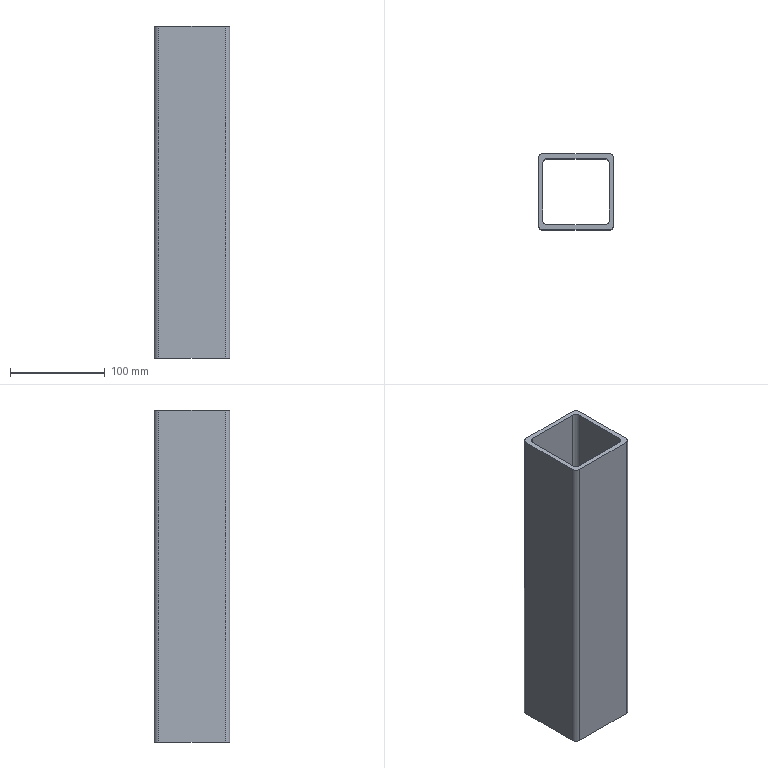Part | SolidWorks | features BaseBody 1 | 1 solid | 18 faces | box 80 x 80 x 350 mm | volume 525000 mm3 | plane 10 | cylinder 8 | commonest cylinder face diameters 10 x8
STEP:
#1=CARTESIAN_POINT('',(-40.,-35.,175.));
#2=VERTEX_POINT('',#1);
#3=CARTESIAN_POINT('',(-35.,-40.,175.));
#4=VERTEX_POINT('',#3);
#5=CARTESIAN_POINT('',(-35.,-35.,175.));
#6=DIRECTION('',(0.,0.,1.));
#7=DIRECTION('',(-1.,0.,0.));
#8=AXIS2_PLACEMENT_3D('',#5,#6,#7);
#9=CIRCLE('',#8,5.);
#10=EDGE_CURVE('',#2,#4,#9,.T.);
#11=ORIENTED_EDGE('',*,*,#10,.T.);
#12=CARTESIAN_POINT('',(35.,-40.,175.));
#13=VERTEX_POINT('',#12);
#14=CARTESIAN_POINT('',(35.,-40.,175.));
#15=DIRECTION('',(1.,0.,0.));
#16=VECTOR('',#15,1000.);
#17=LINE('',#14,#16);
#18=EDGE_CURVE('',#4,#13,#17,.T.);
#19=ORIENTED_EDGE('',*,*,#18,.T.);
#20=CARTESIAN_POINT('',(40.,-35.,175.));
#21=VERTEX_POINT('',#20);
#22=CARTESIAN_POINT('',(35.,-35.,175.));
#23=DIRECTION('',(0.,0.,1.));
#24=DIRECTION('',(1.,0.,0.));
#25=AXIS2_PLACEMENT_3D('',#22,#23,#24);
#26=CIRCLE('',#25,5.);
#27=EDGE_CURVE('',#13,#21,#26,.T.);
#28=ORIENTED_EDGE('',*,*,#27,.T.);
#29=CARTESIAN_POINT('',(40.,35.,175.));
#30=VERTEX_POINT('',#29);
#31=CARTESIAN_POINT('',(40.,-35.,175.));
#32=DIRECTION('',(0.,1.,0.));
#33=VECTOR('',#32,1000.);
#34=LINE('',#31,#33);
#35=EDGE_CURVE('',#21,#30,#34,.T.);
#36=ORIENTED_EDGE('',*,*,#35,.T.);
#37=CARTESIAN_POINT('',(35.,40.,175.));
#38=VERTEX_POINT('',#37);
#39=CARTESIAN_POINT('',(35.,35.,175.));
#40=DIRECTION('',(0.,0.,1.));
#41=DIRECTION('',(1.,0.,0.));
#42=AXIS2_PLACEMENT_3D('',#39,#40,#41);
#43=CIRCLE('',#42,5.);
#44=EDGE_CURVE('',#30,#38,#43,.T.);
#45=ORIENTED_EDGE('',*,*,#44,.T.);
#46=CARTESIAN_POINT('',(-35.,40.,175.));
#47=VERTEX_POINT('',#46);
#48=CARTESIAN_POINT('',(35.,40.,175.));
#49=DIRECTION('',(-1.,0.,0.));
#50=VECTOR('',#49,1000.);
#51=LINE('',#48,#50);
#52=EDGE_CURVE('',#38,#47,#51,.T.);
#53=ORIENTED_EDGE('',*,*,#52,.T.);
#54=CARTESIAN_POINT('',(-40.,35.,175.));
#55=VERTEX_POINT('',#54);
#56=CARTESIAN_POINT('',(-35.,35.,175.));
#57=DIRECTION('',(0.,0.,1.));
#58=DIRECTION('',(1.,0.,0.));
#59=AXIS2_PLACEMENT_3D('',#56,#57,#58);
#60=CIRCLE('',#59,5.);
#61=EDGE_CURVE('',#47,#55,#60,.T.);
#62=ORIENTED_EDGE('',*,*,#61,.T.);
#63=CARTESIAN_POINT('',(-40.,-35.,175.));
#64=DIRECTION('',(0.,-1.,0.));
#65=VECTOR('',#64,1000.);
#66=LINE('',#63,#65);
#67=EDGE_CURVE('',#55,#2,#66,.T.);
#68=ORIENTED_EDGE('',*,*,#67,.T.);
#69=EDGE_LOOP('',(#11,#19,#28,#36,#45,#53,#62,#68));
#70=FACE_OUTER_BOUND('',#69,.T.);
#71=CARTESIAN_POINT('',(-35.,-30.,175.));
#72=VERTEX_POINT('',#71);
#73=CARTESIAN_POINT('',(-30.,-35.,175.));
#74=VERTEX_POINT('',#73);
#75=CARTESIAN_POINT('',(-30.,-30.,175.));
#76=DIRECTION('',(0.,0.,1.));
#77=DIRECTION('',(-1.,0.,0.));
#78=AXIS2_PLACEMENT_3D('',#75,#76,#77);
#79=CIRCLE('',#78,5.);
#80=EDGE_CURVE('',#72,#74,#79,.T.);
#81=ORIENTED_EDGE('',*,*,#80,.F.);
#82=CARTESIAN_POINT('',(-35.,30.,175.));
#83=VERTEX_POINT('',#82);
#84=CARTESIAN_POINT('',(-35.,-30.,175.));
#85=DIRECTION('',(0.,-1.,0.));
#86=VECTOR('',#85,1000.);
#87=LINE('',#84,#86);
#88=EDGE_CURVE('',#83,#72,#87,.T.);
#89=ORIENTED_EDGE('',*,*,#88,.F.);
#90=CARTESIAN_POINT('',(-30.,35.,175.));
#91=VERTEX_POINT('',#90);
#92=CARTESIAN_POINT('',(-30.,30.,175.));
#93=DIRECTION('',(0.,0.,1.));
#94=DIRECTION('',(1.,0.,0.));
#95=AXIS2_PLACEMENT_3D('',#92,#93,#94);
#96=CIRCLE('',#95,5.);
#97=EDGE_CURVE('',#91,#83,#96,.T.);
#98=ORIENTED_EDGE('',*,*,#97,.F.);
#99=CARTESIAN_POINT('',(30.,35.,175.));
#100=VERTEX_POINT('',#99);
#101=CARTESIAN_POINT('',(30.,35.,175.));
#102=DIRECTION('',(-1.,0.,0.));
#103=VECTOR('',#102,1000.);
#104=LINE('',#101,#103);
#105=EDGE_CURVE('',#100,#91,#104,.T.);
#106=ORIENTED_EDGE('',*,*,#105,.F.);
#107=CARTESIAN_POINT('',(35.,30.,175.));
#108=VERTEX_POINT('',#107);
#109=CARTESIAN_POINT('',(30.,30.,175.));
#110=DIRECTION('',(0.,0.,1.));
#111=DIRECTION('',(1.,0.,0.));
#112=AXIS2_PLACEMENT_3D('',#109,#110,#111);
#113=CIRCLE('',#112,5.);
#114=EDGE_CURVE('',#108,#100,#113,.T.);
#115=ORIENTED_EDGE('',*,*,#114,.F.);
#116=CARTESIAN_POINT('',(35.,-30.,175.));
#117=VERTEX_POINT('',#116);
#118=CARTESIAN_POINT('',(35.,-30.,175.));
#119=DIRECTION('',(0.,1.,0.));
#120=VECTOR('',#119,1000.);
#121=LINE('',#118,#120);
#122=EDGE_CURVE('',#117,#108,#121,.T.);
#123=ORIENTED_EDGE('',*,*,#122,.F.);
#124=CARTESIAN_POINT('',(30.,-35.,175.));
#125=VERTEX_POINT('',#124);
#126=CARTESIAN_POINT('',(30.,-30.,175.));
#127=DIRECTION('',(0.,0.,1.));
#128=DIRECTION('',(1.,0.,0.));
#129=AXIS2_PLACEMENT_3D('',#126,#127,#128);
#130=CIRCLE('',#129,5.);
#131=EDGE_CURVE('',#125,#117,#130,.T.);
#132=ORIENTED_EDGE('',*,*,#131,.F.);
#133=CARTESIAN_POINT('',(30.,-35.,175.));
#134=DIRECTION('',(1.,0.,0.));
#135=VECTOR('',#134,1000.);
#136=LINE('',#133,#135);
#137=EDGE_CURVE('',#74,#125,#136,.T.);
#138=ORIENTED_EDGE('',*,*,#137,.F.);
#139=EDGE_LOOP('',(#81,#89,#98,#106,#115,#123,#132,#138));
#140=FACE_BOUND('',#139,.T.);
#141=CARTESIAN_POINT('',(-35.,-35.,175.));
#142=DIRECTION('',(0.,0.,-1.));
#143=DIRECTION('',(-1.,0.,0.));
#144=AXIS2_PLACEMENT_3D('',#141,#142,#143);
#145=PLANE('',#144);
#146=ADVANCED_FACE('',(#70,#140),#145,.F.);
#147=CARTESIAN_POINT('',(-40.,-35.,-175.));
#148=VERTEX_POINT('',#147);
#149=CARTESIAN_POINT('',(-35.,-40.,-175.));
#150=VERTEX_POINT('',#149);
#151=CARTESIAN_POINT('',(-35.,-35.,-175.));
#152=DIRECTION('',(0.,0.,1.));
#153=DIRECTION('',(-1.,0.,0.));
#154=AXIS2_PLACEMENT_3D('',#151,#152,#153);
#155=CIRCLE('',#154,5.);
#156=EDGE_CURVE('',#148,#150,#155,.T.);
#157=ORIENTED_EDGE('',*,*,#156,.F.);
#158=CARTESIAN_POINT('',(-40.,35.,-175.));
#159=VERTEX_POINT('',#158);
#160=CARTESIAN_POINT('',(-40.,-35.,-175.));
#161=DIRECTION('',(0.,-1.,0.));
#162=VECTOR('',#161,1000.);
#163=LINE('',#160,#162);
#164=EDGE_CURVE('',#159,#148,#163,.T.);
#165=ORIENTED_EDGE('',*,*,#164,.F.);
#166=CARTESIAN_POINT('',(-35.,40.,-175.));
#167=VERTEX_POINT('',#166);
#168=CARTESIAN_POINT('',(-35.,35.,-175.));
#169=DIRECTION('',(0.,0.,1.));
#170=DIRECTION('',(1.,0.,0.));
#171=AXIS2_PLACEMENT_3D('',#168,#169,#170);
#172=CIRCLE('',#171,5.);
#173=EDGE_CURVE('',#167,#159,#172,.T.);
#174=ORIENTED_EDGE('',*,*,#173,.F.);
#175=CARTESIAN_POINT('',(35.,40.,-175.));
#176=VERTEX_POINT('',#175);
#177=CARTESIAN_POINT('',(35.,40.,-175.));
#178=DIRECTION('',(-1.,0.,0.));
#179=VECTOR('',#178,1000.);
#180=LINE('',#177,#179);
#181=EDGE_CURVE('',#176,#167,#180,.T.);
#182=ORIENTED_EDGE('',*,*,#181,.F.);
#183=CARTESIAN_POINT('',(40.,35.,-175.));
#184=VERTEX_POINT('',#183);
#185=CARTESIAN_POINT('',(35.,35.,-175.));
#186=DIRECTION('',(0.,0.,1.));
#187=DIRECTION('',(1.,0.,0.));
#188=AXIS2_PLACEMENT_3D('',#185,#186,#187);
#189=CIRCLE('',#188,5.);
#190=EDGE_CURVE('',#184,#176,#189,.T.);
#191=ORIENTED_EDGE('',*,*,#190,.F.);
#192=CARTESIAN_POINT('',(40.,-35.,-175.));
#193=VERTEX_POINT('',#192);
#194=CARTESIAN_POINT('',(40.,-35.,-175.));
#195=DIRECTION('',(0.,1.,0.));
#196=VECTOR('',#195,1000.);
#197=LINE('',#194,#196);
#198=EDGE_CURVE('',#193,#184,#197,.T.);
#199=ORIENTED_EDGE('',*,*,#198,.F.);
#200=CARTESIAN_POINT('',(35.,-40.,-175.));
#201=VERTEX_POINT('',#200);
#202=CARTESIAN_POINT('',(35.,-35.,-175.));
#203=DIRECTION('',(0.,0.,1.));
#204=DIRECTION('',(1.,0.,0.));
#205=AXIS2_PLACEMENT_3D('',#202,#203,#204);
#206=CIRCLE('',#205,5.);
#207=EDGE_CURVE('',#201,#193,#206,.T.);
#208=ORIENTED_EDGE('',*,*,#207,.F.);
#209=CARTESIAN_POINT('',(35.,-40.,-175.));
#210=DIRECTION('',(1.,0.,0.));
#211=VECTOR('',#210,1000.);
#212=LINE('',#209,#211);
#213=EDGE_CURVE('',#150,#201,#212,.T.);
#214=ORIENTED_EDGE('',*,*,#213,.F.);
#215=EDGE_LOOP('',(#157,#165,#174,#182,#191,#199,#208,#214));
#216=FACE_OUTER_BOUND('',#215,.T.);
#217=CARTESIAN_POINT('',(-35.,30.,-175.));
#218=VERTEX_POINT('',#217);
#219=CARTESIAN_POINT('',(-35.,-30.,-175.));
#220=VERTEX_POINT('',#219);
#221=CARTESIAN_POINT('',(-35.,-30.,-175.));
#222=DIRECTION('',(0.,-1.,0.));
#223=VECTOR('',#222,1000.);
#224=LINE('',#221,#223);
#225=EDGE_CURVE('',#218,#220,#224,.T.);
#226=ORIENTED_EDGE('',*,*,#225,.T.);
#227=CARTESIAN_POINT('',(-30.,-35.,-175.));
#228=VERTEX_POINT('',#227);
#229=CARTESIAN_POINT('',(-30.,-30.,-175.));
#230=DIRECTION('',(0.,0.,1.));
#231=DIRECTION('',(-1.,0.,0.));
#232=AXIS2_PLACEMENT_3D('',#229,#230,#231);
#233=CIRCLE('',#232,5.);
#234=EDGE_CURVE('',#220,#228,#233,.T.);
#235=ORIENTED_EDGE('',*,*,#234,.T.);
#236=CARTESIAN_POINT('',(30.,-35.,-175.));
#237=VERTEX_POINT('',#236);
#238=CARTESIAN_POINT('',(30.,-35.,-175.));
#239=DIRECTION('',(1.,0.,0.));
#240=VECTOR('',#239,1000.);
#241=LINE('',#238,#240);
#242=EDGE_CURVE('',#228,#237,#241,.T.);
#243=ORIENTED_EDGE('',*,*,#242,.T.);
#244=CARTESIAN_POINT('',(35.,-30.,-175.));
#245=VERTEX_POINT('',#244);
#246=CARTESIAN_POINT('',(30.,-30.,-175.));
#247=DIRECTION('',(0.,0.,1.));
#248=DIRECTION('',(1.,0.,0.));
#249=AXIS2_PLACEMENT_3D('',#246,#247,#248);
#250=CIRCLE('',#249,5.);
#251=EDGE_CURVE('',#237,#245,#250,.T.);
#252=ORIENTED_EDGE('',*,*,#251,.T.);
#253=CARTESIAN_POINT('',(35.,30.,-175.));
#254=VERTEX_POINT('',#253);
#255=CARTESIAN_POINT('',(35.,-30.,-175.));
#256=DIRECTION('',(0.,1.,0.));
#257=VECTOR('',#256,1000.);
#258=LINE('',#255,#257);
#259=EDGE_CURVE('',#245,#254,#258,.T.);
#260=ORIENTED_EDGE('',*,*,#259,.T.);
#261=CARTESIAN_POINT('',(30.,35.,-175.));
#262=VERTEX_POINT('',#261);
#263=CARTESIAN_POINT('',(30.,30.,-175.));
#264=DIRECTION('',(0.,0.,1.));
#265=DIRECTION('',(1.,0.,0.));
#266=AXIS2_PLACEMENT_3D('',#263,#264,#265);
#267=CIRCLE('',#266,5.);
#268=EDGE_CURVE('',#254,#262,#267,.T.);
#269=ORIENTED_EDGE('',*,*,#268,.T.);
#270=CARTESIAN_POINT('',(-30.,35.,-175.));
#271=VERTEX_POINT('',#270);
#272=CARTESIAN_POINT('',(30.,35.,-175.));
#273=DIRECTION('',(-1.,0.,0.));
#274=VECTOR('',#273,1000.);
#275=LINE('',#272,#274);
#276=EDGE_CURVE('',#262,#271,#275,.T.);
#277=ORIENTED_EDGE('',*,*,#276,.T.);
#278=CARTESIAN_POINT('',(-30.,30.,-175.));
#279=DIRECTION('',(0.,0.,1.));
#280=DIRECTION('',(1.,0.,0.));
#281=AXIS2_PLACEMENT_3D('',#278,#279,#280);
#282=CIRCLE('',#281,5.);
#283=EDGE_CURVE('',#271,#218,#282,.T.);
#284=ORIENTED_EDGE('',*,*,#283,.T.);
#285=EDGE_LOOP('',(#226,#235,#243,#252,#260,#269,#277,#284));
#286=FACE_BOUND('',#285,.T.);
#287=CARTESIAN_POINT('',(-35.,-35.,-175.));
#288=DIRECTION('',(0.,0.,-1.));
#289=DIRECTION('',(-1.,0.,0.));
#290=AXIS2_PLACEMENT_3D('',#287,#288,#289);
#291=PLANE('',#290);
#292=ADVANCED_FACE('',(#216,#286),#291,.T.);
#293=ORIENTED_EDGE('',*,*,#156,.T.);
#294=CARTESIAN_POINT('',(-35.,-40.,175.));
#295=DIRECTION('',(0.,0.,-1.));
#296=VECTOR('',#295,1000.);
#297=LINE('',#294,#296);
#298=EDGE_CURVE('',#4,#150,#297,.T.);
#299=ORIENTED_EDGE('',*,*,#298,.F.);
#300=ORIENTED_EDGE('',*,*,#10,.F.);
#301=CARTESIAN_POINT('',(-40.,-35.,175.));
#302=DIRECTION('',(0.,0.,-1.));
#303=VECTOR('',#302,1000.);
#304=LINE('',#301,#303);
#305=EDGE_CURVE('',#2,#148,#304,.T.);
#306=ORIENTED_EDGE('',*,*,#305,.T.);
#307=EDGE_LOOP('',(#293,#299,#300,#306));
#308=FACE_OUTER_BOUND('',#307,.T.);
#309=CARTESIAN_POINT('',(-35.,-35.,175.));
#310=DIRECTION('',(0.,0.,-1.));
#311=DIRECTION('',(-1.,0.,0.));
#312=AXIS2_PLACEMENT_3D('',#309,#310,#311);
#313=CYLINDRICAL_SURFACE('',#312,5.);
#314=ADVANCED_FACE('',(#308),#313,.T.);
#315=ORIENTED_EDGE('',*,*,#213,.T.);
#316=CARTESIAN_POINT('',(35.,-40.,175.));
#317=DIRECTION('',(0.,0.,-1.));
#318=VECTOR('',#317,1000.);
#319=LINE('',#316,#318);
#320=EDGE_CURVE('',#13,#201,#319,.T.);
#321=ORIENTED_EDGE('',*,*,#320,.F.);
#322=ORIENTED_EDGE('',*,*,#18,.F.);
#323=ORIENTED_EDGE('',*,*,#298,.T.);
#324=EDGE_LOOP('',(#315,#321,#322,#323));
#325=FACE_OUTER_BOUND('',#324,.T.);
#326=CARTESIAN_POINT('',(35.,-40.,175.));
#327=DIRECTION('',(0.,1.,0.));
#328=DIRECTION('',(-1.,0.,0.));
#329=AXIS2_PLACEMENT_3D('',#326,#327,#328);
#330=PLANE('',#329);
#331=ADVANCED_FACE('',(#325),#330,.F.);
#332=ORIENTED_EDGE('',*,*,#207,.T.);
#333=CARTESIAN_POINT('',(40.,-35.,175.));
#334=DIRECTION('',(0.,0.,-1.));
#335=VECTOR('',#334,1000.);
#336=LINE('',#333,#335);
#337=EDGE_CURVE('',#21,#193,#336,.T.);
#338=ORIENTED_EDGE('',*,*,#337,.F.);
#339=ORIENTED_EDGE('',*,*,#27,.F.);
#340=ORIENTED_EDGE('',*,*,#320,.T.);
#341=EDGE_LOOP('',(#332,#338,#339,#340));
#342=FACE_OUTER_BOUND('',#341,.T.);
#343=CARTESIAN_POINT('',(35.,-35.,175.));
#344=DIRECTION('',(0.,0.,-1.));
#345=DIRECTION('',(-1.,0.,0.));
#346=AXIS2_PLACEMENT_3D('',#343,#344,#345);
#347=CYLINDRICAL_SURFACE('',#346,5.);
#348=ADVANCED_FACE('',(#342),#347,.T.);
#349=ORIENTED_EDGE('',*,*,#198,.T.);
#350=CARTESIAN_POINT('',(40.,35.,175.));
#351=DIRECTION('',(0.,0.,-1.));
#352=VECTOR('',#351,1000.);
#353=LINE('',#350,#352);
#354=EDGE_CURVE('',#30,#184,#353,.T.);
#355=ORIENTED_EDGE('',*,*,#354,.F.);
#356=ORIENTED_EDGE('',*,*,#35,.F.);
#357=ORIENTED_EDGE('',*,*,#337,.T.);
#358=EDGE_LOOP('',(#349,#355,#356,#357));
#359=FACE_OUTER_BOUND('',#358,.T.);
#360=CARTESIAN_POINT('',(40.,-35.,175.));
#361=DIRECTION('',(-1.,0.,0.));
#362=DIRECTION('',(0.,-1.,0.));
#363=AXIS2_PLACEMENT_3D('',#360,#361,#362);
#364=PLANE('',#363);
#365=ADVANCED_FACE('',(#359),#364,.F.);
#366=ORIENTED_EDGE('',*,*,#190,.T.);
#367=CARTESIAN_POINT('',(35.,40.,175.));
#368=DIRECTION('',(0.,0.,-1.));
#369=VECTOR('',#368,1000.);
#370=LINE('',#367,#369);
#371=EDGE_CURVE('',#38,#176,#370,.T.);
#372=ORIENTED_EDGE('',*,*,#371,.F.);
#373=ORIENTED_EDGE('',*,*,#44,.F.);
#374=ORIENTED_EDGE('',*,*,#354,.T.);
#375=EDGE_LOOP('',(#366,#372,#373,#374));
#376=FACE_OUTER_BOUND('',#375,.T.);
#377=CARTESIAN_POINT('',(35.,35.,175.));
#378=DIRECTION('',(0.,0.,-1.));
#379=DIRECTION('',(-1.,0.,0.));
#380=AXIS2_PLACEMENT_3D('',#377,#378,#379);
#381=CYLINDRICAL_SURFACE('',#380,5.);
#382=ADVANCED_FACE('',(#376),#381,.T.);
#383=ORIENTED_EDGE('',*,*,#181,.T.);
#384=CARTESIAN_POINT('',(-35.,40.,175.));
#385=DIRECTION('',(0.,0.,-1.));
#386=VECTOR('',#385,1000.);
#387=LINE('',#384,#386);
#388=EDGE_CURVE('',#47,#167,#387,.T.);
#389=ORIENTED_EDGE('',*,*,#388,.F.);
#390=ORIENTED_EDGE('',*,*,#52,.F.);
#391=ORIENTED_EDGE('',*,*,#371,.T.);
#392=EDGE_LOOP('',(#383,#389,#390,#391));
#393=FACE_OUTER_BOUND('',#392,.T.);
#394=CARTESIAN_POINT('',(35.,40.,175.));
#395=DIRECTION('',(0.,-1.,0.));
#396=DIRECTION('',(1.,0.,0.));
#397=AXIS2_PLACEMENT_3D('',#394,#395,#396);
#398=PLANE('',#397);
#399=ADVANCED_FACE('',(#393),#398,.F.);
#400=ORIENTED_EDGE('',*,*,#173,.T.);
#401=CARTESIAN_POINT('',(-40.,35.,175.));
#402=DIRECTION('',(0.,0.,-1.));
#403=VECTOR('',#402,1000.);
#404=LINE('',#401,#403);
#405=EDGE_CURVE('',#55,#159,#404,.T.);
#406=ORIENTED_EDGE('',*,*,#405,.F.);
#407=ORIENTED_EDGE('',*,*,#61,.F.);
#408=ORIENTED_EDGE('',*,*,#388,.T.);
#409=EDGE_LOOP('',(#400,#406,#407,#408));
#410=FACE_OUTER_BOUND('',#409,.T.);
#411=CARTESIAN_POINT('',(-35.,35.,175.));
#412=DIRECTION('',(0.,0.,-1.));
#413=DIRECTION('',(-1.,0.,0.));
#414=AXIS2_PLACEMENT_3D('',#411,#412,#413);
#415=CYLINDRICAL_SURFACE('',#414,5.);
#416=ADVANCED_FACE('',(#410),#415,.T.);
#417=ORIENTED_EDGE('',*,*,#164,.T.);
#418=ORIENTED_EDGE('',*,*,#305,.F.);
#419=ORIENTED_EDGE('',*,*,#67,.F.);
#420=ORIENTED_EDGE('',*,*,#405,.T.);
#421=EDGE_LOOP('',(#417,#418,#419,#420));
#422=FACE_OUTER_BOUND('',#421,.T.);
#423=CARTESIAN_POINT('',(-40.,-35.,175.));
#424=DIRECTION('',(1.,0.,0.));
#425=DIRECTION('',(0.,1.,0.));
#426=AXIS2_PLACEMENT_3D('',#423,#424,#425);
#427=PLANE('',#426);
#428=ADVANCED_FACE('',(#422),#427,.F.);
#429=ORIENTED_EDGE('',*,*,#234,.F.);
#430=CARTESIAN_POINT('',(-35.,-30.,175.));
#431=DIRECTION('',(0.,0.,-1.));
#432=VECTOR('',#431,1000.);
#433=LINE('',#430,#432);
#434=EDGE_CURVE('',#72,#220,#433,.T.);
#435=ORIENTED_EDGE('',*,*,#434,.F.);
#436=ORIENTED_EDGE('',*,*,#80,.T.);
#437=CARTESIAN_POINT('',(-30.,-35.,175.));
#438=DIRECTION('',(0.,0.,-1.));
#439=VECTOR('',#438,1000.);
#440=LINE('',#437,#439);
#441=EDGE_CURVE('',#74,#228,#440,.T.);
#442=ORIENTED_EDGE('',*,*,#441,.T.);
#443=EDGE_LOOP('',(#429,#435,#436,#442));
#444=FACE_OUTER_BOUND('',#443,.T.);
#445=CARTESIAN_POINT('',(-30.,-30.,175.));
#446=DIRECTION('',(0.,0.,-1.));
#447=DIRECTION('',(-1.,0.,0.));
#448=AXIS2_PLACEMENT_3D('',#445,#446,#447);
#449=CYLINDRICAL_SURFACE('',#448,5.);
#450=ADVANCED_FACE('',(#444),#449,.F.);
#451=ORIENTED_EDGE('',*,*,#242,.F.);
#452=ORIENTED_EDGE('',*,*,#441,.F.);
#453=ORIENTED_EDGE('',*,*,#137,.T.);
#454=CARTESIAN_POINT('',(30.,-35.,175.));
#455=DIRECTION('',(0.,0.,-1.));
#456=VECTOR('',#455,1000.);
#457=LINE('',#454,#456);
#458=EDGE_CURVE('',#125,#237,#457,.T.);
#459=ORIENTED_EDGE('',*,*,#458,.T.);
#460=EDGE_LOOP('',(#451,#452,#453,#459));
#461=FACE_OUTER_BOUND('',#460,.T.);
#462=CARTESIAN_POINT('',(30.,-35.,175.));
#463=DIRECTION('',(0.,1.,0.));
#464=DIRECTION('',(-1.,0.,0.));
#465=AXIS2_PLACEMENT_3D('',#462,#463,#464);
#466=PLANE('',#465);
#467=ADVANCED_FACE('',(#461),#466,.T.);
#468=ORIENTED_EDGE('',*,*,#251,.F.);
#469=ORIENTED_EDGE('',*,*,#458,.F.);
#470=ORIENTED_EDGE('',*,*,#131,.T.);
#471=CARTESIAN_POINT('',(35.,-30.,175.));
#472=DIRECTION('',(0.,0.,-1.));
#473=VECTOR('',#472,1000.);
#474=LINE('',#471,#473);
#475=EDGE_CURVE('',#117,#245,#474,.T.);
#476=ORIENTED_EDGE('',*,*,#475,.T.);
#477=EDGE_LOOP('',(#468,#469,#470,#476));
#478=FACE_OUTER_BOUND('',#477,.T.);
#479=CARTESIAN_POINT('',(30.,-30.,175.));
#480=DIRECTION('',(0.,0.,-1.));
#481=DIRECTION('',(-1.,0.,0.));
#482=AXIS2_PLACEMENT_3D('',#479,#480,#481);
#483=CYLINDRICAL_SURFACE('',#482,5.);
#484=ADVANCED_FACE('',(#478),#483,.F.);
#485=ORIENTED_EDGE('',*,*,#259,.F.);
#486=ORIENTED_EDGE('',*,*,#475,.F.);
#487=ORIENTED_EDGE('',*,*,#122,.T.);
#488=CARTESIAN_POINT('',(35.,30.,175.));
#489=DIRECTION('',(0.,0.,-1.));
#490=VECTOR('',#489,1000.);
#491=LINE('',#488,#490);
#492=EDGE_CURVE('',#108,#254,#491,.T.);
#493=ORIENTED_EDGE('',*,*,#492,.T.);
#494=EDGE_LOOP('',(#485,#486,#487,#493));
#495=FACE_OUTER_BOUND('',#494,.T.);
#496=CARTESIAN_POINT('',(35.,-30.,175.));
#497=DIRECTION('',(-1.,0.,0.));
#498=DIRECTION('',(0.,0.,1.));
#499=AXIS2_PLACEMENT_3D('',#496,#497,#498);
#500=PLANE('',#499);
#501=ADVANCED_FACE('',(#495),#500,.T.);
#502=ORIENTED_EDGE('',*,*,#268,.F.);
#503=ORIENTED_EDGE('',*,*,#492,.F.);
#504=ORIENTED_EDGE('',*,*,#114,.T.);
#505=CARTESIAN_POINT('',(30.,35.,175.));
#506=DIRECTION('',(0.,0.,-1.));
#507=VECTOR('',#506,1000.);
#508=LINE('',#505,#507);
#509=EDGE_CURVE('',#100,#262,#508,.T.);
#510=ORIENTED_EDGE('',*,*,#509,.T.);
#511=EDGE_LOOP('',(#502,#503,#504,#510));
#512=FACE_OUTER_BOUND('',#511,.T.);
#513=CARTESIAN_POINT('',(30.,30.,175.));
#514=DIRECTION('',(0.,0.,-1.));
#515=DIRECTION('',(-1.,0.,0.));
#516=AXIS2_PLACEMENT_3D('',#513,#514,#515);
#517=CYLINDRICAL_SURFACE('',#516,5.);
#518=ADVANCED_FACE('',(#512),#517,.F.);
#519=ORIENTED_EDGE('',*,*,#276,.F.);
#520=ORIENTED_EDGE('',*,*,#509,.F.);
#521=ORIENTED_EDGE('',*,*,#105,.T.);
#522=CARTESIAN_POINT('',(-30.,35.,175.));
#523=DIRECTION('',(0.,0.,-1.));
#524=VECTOR('',#523,1000.);
#525=LINE('',#522,#524);
#526=EDGE_CURVE('',#91,#271,#525,.T.);
#527=ORIENTED_EDGE('',*,*,#526,.T.);
#528=EDGE_LOOP('',(#519,#520,#521,#527));
#529=FACE_OUTER_BOUND('',#528,.T.);
#530=CARTESIAN_POINT('',(30.,35.,175.));
#531=DIRECTION('',(0.,-1.,0.));
#532=DIRECTION('',(1.,0.,0.));
#533=AXIS2_PLACEMENT_3D('',#530,#531,#532);
#534=PLANE('',#533);
#535=ADVANCED_FACE('',(#529),#534,.T.);
#536=ORIENTED_EDGE('',*,*,#283,.F.);
#537=ORIENTED_EDGE('',*,*,#526,.F.);
#538=ORIENTED_EDGE('',*,*,#97,.T.);
#539=CARTESIAN_POINT('',(-35.,30.,175.));
#540=DIRECTION('',(0.,0.,-1.));
#541=VECTOR('',#540,1000.);
#542=LINE('',#539,#541);
#543=EDGE_CURVE('',#83,#218,#542,.T.);
#544=ORIENTED_EDGE('',*,*,#543,.T.);
#545=EDGE_LOOP('',(#536,#537,#538,#544));
#546=FACE_OUTER_BOUND('',#545,.T.);
#547=CARTESIAN_POINT('',(-30.,30.,175.));
#548=DIRECTION('',(0.,0.,-1.));
#549=DIRECTION('',(-1.,0.,0.));
#550=AXIS2_PLACEMENT_3D('',#547,#548,#549);
#551=CYLINDRICAL_SURFACE('',#550,5.);
#552=ADVANCED_FACE('',(#546),#551,.F.);
#553=ORIENTED_EDGE('',*,*,#225,.F.);
#554=ORIENTED_EDGE('',*,*,#543,.F.);
#555=ORIENTED_EDGE('',*,*,#88,.T.);
#556=ORIENTED_EDGE('',*,*,#434,.T.);
#557=EDGE_LOOP('',(#553,#554,#555,#556));
#558=FACE_OUTER_BOUND('',#557,.T.);
#559=CARTESIAN_POINT('',(-35.,-30.,175.));
#560=DIRECTION('',(1.,0.,0.));
#561=DIRECTION('',(0.,0.,-1.));
#562=AXIS2_PLACEMENT_3D('',#559,#560,#561);
#563=PLANE('',#562);
#564=ADVANCED_FACE('',(#558),#563,.T.);
#565=CLOSED_SHELL('',(#146,#292,#314,#331,#348,#365,#382,#399,#416,#428,#450,#467,#484,#501,#518,#535,#552,#564));
#566=MANIFOLD_SOLID_BREP('',#565);
#567=CARTESIAN_POINT('',(0.,0.,0.));
#568=DIRECTION('',(0.,0.,1.));
#569=DIRECTION('',(1.,0.,0.));
#570=AXIS2_PLACEMENT_3D('',#567,#568,#569);
#571=(LENGTH_UNIT()NAMED_UNIT(*)SI_UNIT(.MILLI.,.METRE.));
#572=UNCERTAINTY_MEASURE_WITH_UNIT(LENGTH_MEASURE(0.00001),#571,'','');
#573=(NAMED_UNIT(*)PLANE_ANGLE_UNIT()SI_UNIT($,.RADIAN.));
#574=(NAMED_UNIT(*)SI_UNIT($,.STERADIAN.)SOLID_ANGLE_UNIT());
#575=(GEOMETRIC_REPRESENTATION_CONTEXT(3)GLOBAL_UNCERTAINTY_ASSIGNED_CONTEXT((#572))GLOBAL_UNIT_ASSIGNED_CONTEXT((#571,#573,#574))REPRESENTATION_CONTEXT('',''));
#576=ADVANCED_BREP_SHAPE_REPRESENTATION('',(#566,#570),#575);